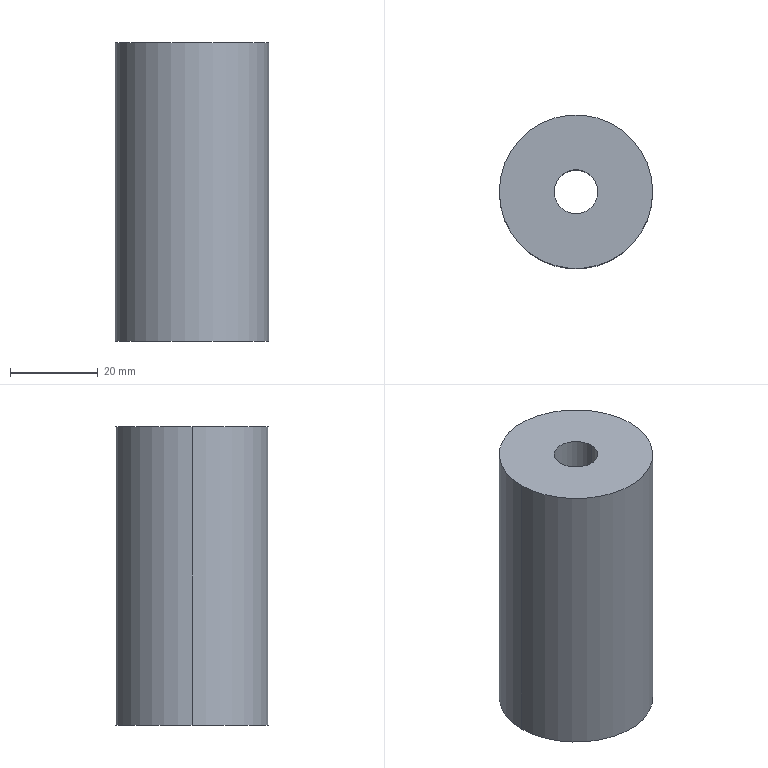Part | STEP file | 1 solid | 6 faces | box 35 x 35 x 68 mm | volume 60083 mm3 | cylinder 4 | plane 2 | commonest cylinder face diameters 10 x2 35 x2
STEP:
#1=CARTESIAN_POINT('',(0.,0.,0.));
#2=DIRECTION('',(0.,0.,1.));
#3=DIRECTION('',(1.,0.,0.));
#4=AXIS2_PLACEMENT_3D('',#1,#2,#3);
#5=CARTESIAN_POINT('',(194.63,-201.166,-34.));
#6=VERTEX_POINT('',#5);
#7=CARTESIAN_POINT('',(159.63,-201.166,-34.));
#8=VERTEX_POINT('',#7);
#9=CARTESIAN_POINT('',(177.13,-201.166,-34.));
#10=DIRECTION('',(0.,0.,1.));
#11=DIRECTION('',(1.,0.,0.));
#12=AXIS2_PLACEMENT_3D('',#9,#10,#11);
#13=CIRCLE('',#12,17.5);
#14=CARTESIAN_POINT('',(177.13,-201.166,0.));
#15=DIRECTION('',(0.,0.,1.));
#16=DIRECTION('',(1.,0.,0.));
#17=AXIS2_PLACEMENT_3D('',#14,#15,#16);
#18=CYLINDRICAL_SURFACE('',#17,17.5);
#19=CARTESIAN_POINT('',(0.,-34.));
#20=DIRECTION('',(1.,0.));
#21=VECTOR('',#20,1.);
#22=LINE('',#19,#21);
#23=(GEOMETRIC_REPRESENTATION_CONTEXT(2)PARAMETRIC_REPRESENTATION_CONTEXT()REPRESENTATION_CONTEXT('',''));
#24=DEFINITIONAL_REPRESENTATION('',(#22),#23);
#25=PCURVE('',#18,#24);
#26=CARTESIAN_POINT('',(177.13,-201.166,-34.));
#27=DIRECTION('',(0.,0.,1.));
#28=DIRECTION('',(1.,0.,0.));
#29=AXIS2_PLACEMENT_3D('',#26,#27,#28);
#30=PLANE('',#29);
#31=CARTESIAN_POINT('',(0.,0.));
#32=DIRECTION('',(1.,0.));
#33=AXIS2_PLACEMENT_2D('',#31,#32);
#34=CIRCLE('',#33,17.5);
#35=(GEOMETRIC_REPRESENTATION_CONTEXT(2)PARAMETRIC_REPRESENTATION_CONTEXT()REPRESENTATION_CONTEXT('',''));
#36=DEFINITIONAL_REPRESENTATION('',(#34),#35);
#37=PCURVE('',#30,#36);
#38=SURFACE_CURVE('',#13,(#25,#37),.PCURVE_S1.);
#39=EDGE_CURVE('',#6,#8,#38,.T.);
#40=ORIENTED_EDGE('',*,*,#39,.T.);
#41=CARTESIAN_POINT('',(159.63,-201.166,34.));
#42=VERTEX_POINT('',#41);
#43=CARTESIAN_POINT('',(159.63,-201.166,0.));
#44=DIRECTION('',(0.,0.,1.));
#45=VECTOR('',#44,1.);
#46=LINE('',#43,#45);
#47=CARTESIAN_POINT('',(3.142,0.));
#48=DIRECTION('',(0.,1.));
#49=VECTOR('',#48,1.);
#50=LINE('',#47,#49);
#51=(GEOMETRIC_REPRESENTATION_CONTEXT(2)PARAMETRIC_REPRESENTATION_CONTEXT()REPRESENTATION_CONTEXT('',''));
#52=DEFINITIONAL_REPRESENTATION('',(#50),#51);
#53=PCURVE('',#18,#52);
#54=CARTESIAN_POINT('',(177.13,-201.166,0.));
#55=DIRECTION('',(0.,0.,1.));
#56=DIRECTION('',(1.,0.,0.));
#57=AXIS2_PLACEMENT_3D('',#54,#55,#56);
#58=CYLINDRICAL_SURFACE('',#57,17.5);
#59=CARTESIAN_POINT('',(3.142,0.));
#60=DIRECTION('',(0.,1.));
#61=VECTOR('',#60,1.);
#62=LINE('',#59,#61);
#63=(GEOMETRIC_REPRESENTATION_CONTEXT(2)PARAMETRIC_REPRESENTATION_CONTEXT()REPRESENTATION_CONTEXT('',''));
#64=DEFINITIONAL_REPRESENTATION('',(#62),#63);
#65=PCURVE('',#58,#64);
#66=SURFACE_CURVE('',#46,(#53,#65),.PCURVE_S1.);
#67=EDGE_CURVE('',#8,#42,#66,.T.);
#68=ORIENTED_EDGE('',*,*,#67,.T.);
#69=CARTESIAN_POINT('',(194.63,-201.166,34.));
#70=VERTEX_POINT('',#69);
#71=CARTESIAN_POINT('',(177.13,-201.166,34.));
#72=DIRECTION('',(0.,0.,-1.));
#73=DIRECTION('',(1.,0.,0.));
#74=AXIS2_PLACEMENT_3D('',#71,#72,#73);
#75=CIRCLE('',#74,17.5);
#76=CARTESIAN_POINT('',(6.283,34.));
#77=DIRECTION('',(-1.,0.));
#78=VECTOR('',#77,1.);
#79=LINE('',#76,#78);
#80=(GEOMETRIC_REPRESENTATION_CONTEXT(2)PARAMETRIC_REPRESENTATION_CONTEXT()REPRESENTATION_CONTEXT('',''));
#81=DEFINITIONAL_REPRESENTATION('',(#79),#80);
#82=PCURVE('',#18,#81);
#83=CARTESIAN_POINT('',(177.13,-201.166,34.));
#84=DIRECTION('',(0.,0.,1.));
#85=DIRECTION('',(1.,0.,0.));
#86=AXIS2_PLACEMENT_3D('',#83,#84,#85);
#87=PLANE('',#86);
#88=CARTESIAN_POINT('',(17.5,0.));
#89=CARTESIAN_POINT('',(17.5,-30.311));
#90=CARTESIAN_POINT('',(-8.75,-15.155));
#91=CARTESIAN_POINT('',(-35.,0.));
#92=CARTESIAN_POINT('',(-8.75,15.155));
#93=CARTESIAN_POINT('',(17.5,30.311));
#94=CARTESIAN_POINT('',(17.5,0.));
#95=(BOUNDED_CURVE()B_SPLINE_CURVE(2,(#88,#89,#90,#91,#92,#93,#94),.UNSPECIFIED.,.T.,.F.)B_SPLINE_CURVE_WITH_KNOTS((1,2,2,2,2,1),(-2.094,0.,2.094,4.189,6.283,8.378),.UNSPECIFIED.)CURVE()GEOMETRIC_REPRESENTATION_ITEM()RATIONAL_B_SPLINE_CURVE((1.,0.5,1.,0.5,1.,0.5,1.))REPRESENTATION_ITEM(''));
#96=(GEOMETRIC_REPRESENTATION_CONTEXT(2)PARAMETRIC_REPRESENTATION_CONTEXT()REPRESENTATION_CONTEXT('',''));
#97=DEFINITIONAL_REPRESENTATION('',(#95),#96);
#98=PCURVE('',#87,#97);
#99=SURFACE_CURVE('',#75,(#82,#98),.PCURVE_S1.);
#100=EDGE_CURVE('',#42,#70,#99,.T.);
#101=ORIENTED_EDGE('',*,*,#100,.T.);
#102=CARTESIAN_POINT('',(194.63,-201.166,0.));
#103=DIRECTION('',(0.,0.,1.));
#104=VECTOR('',#103,1.);
#105=LINE('',#102,#104);
#106=CARTESIAN_POINT('',(0.,0.));
#107=DIRECTION('',(0.,1.));
#108=VECTOR('',#107,1.);
#109=LINE('',#106,#108);
#110=(GEOMETRIC_REPRESENTATION_CONTEXT(2)PARAMETRIC_REPRESENTATION_CONTEXT()REPRESENTATION_CONTEXT('',''));
#111=DEFINITIONAL_REPRESENTATION('',(#109),#110);
#112=PCURVE('',#18,#111);
#113=CARTESIAN_POINT('',(6.283,0.));
#114=DIRECTION('',(0.,1.));
#115=VECTOR('',#114,1.);
#116=LINE('',#113,#115);
#117=(GEOMETRIC_REPRESENTATION_CONTEXT(2)PARAMETRIC_REPRESENTATION_CONTEXT()REPRESENTATION_CONTEXT('',''));
#118=DEFINITIONAL_REPRESENTATION('',(#116),#117);
#119=PCURVE('',#58,#118);
#120=SURFACE_CURVE('',#105,(#112,#119),.PCURVE_S1.);
#121=EDGE_CURVE('',#6,#70,#120,.T.);
#122=ORIENTED_EDGE('',*,*,#121,.F.);
#123=EDGE_LOOP('',(#40,#68,#101,#122));
#124=FACE_BOUND('',#123,.T.);
#125=ADVANCED_FACE('',(#124),#18,.T.);
#126=CARTESIAN_POINT('',(182.13,-201.166,-34.));
#127=VERTEX_POINT('',#126);
#128=CARTESIAN_POINT('',(182.13,-201.166,34.));
#129=VERTEX_POINT('',#128);
#130=CARTESIAN_POINT('',(182.13,-201.166,0.));
#131=DIRECTION('',(0.,0.,1.));
#132=VECTOR('',#131,1.);
#133=LINE('',#130,#132);
#134=CARTESIAN_POINT('',(177.13,-201.166,0.));
#135=DIRECTION('',(0.,0.,1.));
#136=DIRECTION('',(1.,0.,0.));
#137=AXIS2_PLACEMENT_3D('',#134,#135,#136);
#138=CYLINDRICAL_SURFACE('',#137,5.);
#139=CARTESIAN_POINT('',(6.283,0.));
#140=DIRECTION('',(0.,1.));
#141=VECTOR('',#140,1.);
#142=LINE('',#139,#141);
#143=(GEOMETRIC_REPRESENTATION_CONTEXT(2)PARAMETRIC_REPRESENTATION_CONTEXT()REPRESENTATION_CONTEXT('',''));
#144=DEFINITIONAL_REPRESENTATION('',(#142),#143);
#145=PCURVE('',#138,#144);
#146=CARTESIAN_POINT('',(177.13,-201.166,0.));
#147=DIRECTION('',(0.,0.,1.));
#148=DIRECTION('',(1.,0.,0.));
#149=AXIS2_PLACEMENT_3D('',#146,#147,#148);
#150=CYLINDRICAL_SURFACE('',#149,5.);
#151=CARTESIAN_POINT('',(0.,0.));
#152=DIRECTION('',(0.,1.));
#153=VECTOR('',#152,1.);
#154=LINE('',#151,#153);
#155=(GEOMETRIC_REPRESENTATION_CONTEXT(2)PARAMETRIC_REPRESENTATION_CONTEXT()REPRESENTATION_CONTEXT('',''));
#156=DEFINITIONAL_REPRESENTATION('',(#154),#155);
#157=PCURVE('',#150,#156);
#158=SURFACE_CURVE('',#133,(#145,#157),.PCURVE_S1.);
#159=EDGE_CURVE('',#127,#129,#158,.T.);
#160=ORIENTED_EDGE('',*,*,#159,.T.);
#161=CARTESIAN_POINT('',(172.13,-201.166,34.));
#162=VERTEX_POINT('',#161);
#163=CARTESIAN_POINT('',(177.13,-201.166,34.));
#164=DIRECTION('',(0.,0.,-1.));
#165=DIRECTION('',(1.,0.,0.));
#166=AXIS2_PLACEMENT_3D('',#163,#164,#165);
#167=CIRCLE('',#166,5.);
#168=CARTESIAN_POINT('',(6.283,34.));
#169=DIRECTION('',(-1.,0.));
#170=VECTOR('',#169,1.);
#171=LINE('',#168,#170);
#172=(GEOMETRIC_REPRESENTATION_CONTEXT(2)PARAMETRIC_REPRESENTATION_CONTEXT()REPRESENTATION_CONTEXT('',''));
#173=DEFINITIONAL_REPRESENTATION('',(#171),#172);
#174=PCURVE('',#138,#173);
#175=CARTESIAN_POINT('',(5.,0.));
#176=CARTESIAN_POINT('',(5.,-8.66));
#177=CARTESIAN_POINT('',(-2.5,-4.33));
#178=CARTESIAN_POINT('',(-10.,0.));
#179=CARTESIAN_POINT('',(-2.5,4.33));
#180=CARTESIAN_POINT('',(5.,8.66));
#181=CARTESIAN_POINT('',(5.,0.));
#182=(BOUNDED_CURVE()B_SPLINE_CURVE(2,(#175,#176,#177,#178,#179,#180,#181),.UNSPECIFIED.,.T.,.F.)B_SPLINE_CURVE_WITH_KNOTS((1,2,2,2,2,1),(-2.094,0.,2.094,4.189,6.283,8.378),.UNSPECIFIED.)CURVE()GEOMETRIC_REPRESENTATION_ITEM()RATIONAL_B_SPLINE_CURVE((1.,0.5,1.,0.5,1.,0.5,1.))REPRESENTATION_ITEM(''));
#183=(GEOMETRIC_REPRESENTATION_CONTEXT(2)PARAMETRIC_REPRESENTATION_CONTEXT()REPRESENTATION_CONTEXT('',''));
#184=DEFINITIONAL_REPRESENTATION('',(#182),#183);
#185=PCURVE('',#87,#184);
#186=SURFACE_CURVE('',#167,(#174,#185),.PCURVE_S1.);
#187=EDGE_CURVE('',#129,#162,#186,.T.);
#188=ORIENTED_EDGE('',*,*,#187,.T.);
#189=CARTESIAN_POINT('',(172.13,-201.166,-34.));
#190=VERTEX_POINT('',#189);
#191=CARTESIAN_POINT('',(172.13,-201.166,0.));
#192=DIRECTION('',(0.,0.,1.));
#193=VECTOR('',#192,1.);
#194=LINE('',#191,#193);
#195=CARTESIAN_POINT('',(3.142,0.));
#196=DIRECTION('',(0.,1.));
#197=VECTOR('',#196,1.);
#198=LINE('',#195,#197);
#199=(GEOMETRIC_REPRESENTATION_CONTEXT(2)PARAMETRIC_REPRESENTATION_CONTEXT()REPRESENTATION_CONTEXT('',''));
#200=DEFINITIONAL_REPRESENTATION('',(#198),#199);
#201=PCURVE('',#138,#200);
#202=CARTESIAN_POINT('',(3.142,0.));
#203=DIRECTION('',(0.,1.));
#204=VECTOR('',#203,1.);
#205=LINE('',#202,#204);
#206=(GEOMETRIC_REPRESENTATION_CONTEXT(2)PARAMETRIC_REPRESENTATION_CONTEXT()REPRESENTATION_CONTEXT('',''));
#207=DEFINITIONAL_REPRESENTATION('',(#205),#206);
#208=PCURVE('',#150,#207);
#209=SURFACE_CURVE('',#194,(#201,#208),.PCURVE_S1.);
#210=EDGE_CURVE('',#190,#162,#209,.T.);
#211=ORIENTED_EDGE('',*,*,#210,.F.);
#212=CARTESIAN_POINT('',(177.13,-201.166,-34.));
#213=DIRECTION('',(0.,0.,-1.));
#214=DIRECTION('',(1.,0.,0.));
#215=AXIS2_PLACEMENT_3D('',#212,#213,#214);
#216=CIRCLE('',#215,5.);
#217=CARTESIAN_POINT('',(6.283,-34.));
#218=DIRECTION('',(-1.,0.));
#219=VECTOR('',#218,1.);
#220=LINE('',#217,#219);
#221=(GEOMETRIC_REPRESENTATION_CONTEXT(2)PARAMETRIC_REPRESENTATION_CONTEXT()REPRESENTATION_CONTEXT('',''));
#222=DEFINITIONAL_REPRESENTATION('',(#220),#221);
#223=PCURVE('',#138,#222);
#224=CARTESIAN_POINT('',(5.,0.));
#225=CARTESIAN_POINT('',(5.,-8.66));
#226=CARTESIAN_POINT('',(-2.5,-4.33));
#227=CARTESIAN_POINT('',(-10.,0.));
#228=CARTESIAN_POINT('',(-2.5,4.33));
#229=CARTESIAN_POINT('',(5.,8.66));
#230=CARTESIAN_POINT('',(5.,0.));
#231=(BOUNDED_CURVE()B_SPLINE_CURVE(2,(#224,#225,#226,#227,#228,#229,#230),.UNSPECIFIED.,.T.,.F.)B_SPLINE_CURVE_WITH_KNOTS((1,2,2,2,2,1),(-2.094,0.,2.094,4.189,6.283,8.378),.UNSPECIFIED.)CURVE()GEOMETRIC_REPRESENTATION_ITEM()RATIONAL_B_SPLINE_CURVE((1.,0.5,1.,0.5,1.,0.5,1.))REPRESENTATION_ITEM(''));
#232=(GEOMETRIC_REPRESENTATION_CONTEXT(2)PARAMETRIC_REPRESENTATION_CONTEXT()REPRESENTATION_CONTEXT('',''));
#233=DEFINITIONAL_REPRESENTATION('',(#231),#232);
#234=PCURVE('',#30,#233);
#235=SURFACE_CURVE('',#216,(#223,#234),.PCURVE_S1.);
#236=EDGE_CURVE('',#127,#190,#235,.T.);
#237=ORIENTED_EDGE('',*,*,#236,.F.);
#238=EDGE_LOOP('',(#160,#188,#211,#237));
#239=FACE_BOUND('',#238,.F.);
#240=ADVANCED_FACE('',(#239),#138,.F.);
#241=ORIENTED_EDGE('',*,*,#67,.F.);
#242=CARTESIAN_POINT('',(177.13,-201.166,-34.));
#243=DIRECTION('',(0.,0.,1.));
#244=DIRECTION('',(1.,0.,0.));
#245=AXIS2_PLACEMENT_3D('',#242,#243,#244);
#246=CIRCLE('',#245,17.5);
#247=CARTESIAN_POINT('',(0.,-34.));
#248=DIRECTION('',(1.,0.));
#249=VECTOR('',#248,1.);
#250=LINE('',#247,#249);
#251=(GEOMETRIC_REPRESENTATION_CONTEXT(2)PARAMETRIC_REPRESENTATION_CONTEXT()REPRESENTATION_CONTEXT('',''));
#252=DEFINITIONAL_REPRESENTATION('',(#250),#251);
#253=PCURVE('',#58,#252);
#254=CARTESIAN_POINT('',(0.,0.));
#255=DIRECTION('',(1.,0.));
#256=AXIS2_PLACEMENT_2D('',#254,#255);
#257=CIRCLE('',#256,17.5);
#258=(GEOMETRIC_REPRESENTATION_CONTEXT(2)PARAMETRIC_REPRESENTATION_CONTEXT()REPRESENTATION_CONTEXT('',''));
#259=DEFINITIONAL_REPRESENTATION('',(#257),#258);
#260=PCURVE('',#30,#259);
#261=SURFACE_CURVE('',#246,(#253,#260),.PCURVE_S1.);
#262=EDGE_CURVE('',#8,#6,#261,.T.);
#263=ORIENTED_EDGE('',*,*,#262,.T.);
#264=ORIENTED_EDGE('',*,*,#121,.T.);
#265=CARTESIAN_POINT('',(177.13,-201.166,34.));
#266=DIRECTION('',(0.,0.,-1.));
#267=DIRECTION('',(1.,0.,0.));
#268=AXIS2_PLACEMENT_3D('',#265,#266,#267);
#269=CIRCLE('',#268,17.5);
#270=CARTESIAN_POINT('',(6.283,34.));
#271=DIRECTION('',(-1.,0.));
#272=VECTOR('',#271,1.);
#273=LINE('',#270,#272);
#274=(GEOMETRIC_REPRESENTATION_CONTEXT(2)PARAMETRIC_REPRESENTATION_CONTEXT()REPRESENTATION_CONTEXT('',''));
#275=DEFINITIONAL_REPRESENTATION('',(#273),#274);
#276=PCURVE('',#58,#275);
#277=CARTESIAN_POINT('',(17.5,0.));
#278=CARTESIAN_POINT('',(17.5,-30.311));
#279=CARTESIAN_POINT('',(-8.75,-15.155));
#280=CARTESIAN_POINT('',(-35.,0.));
#281=CARTESIAN_POINT('',(-8.75,15.155));
#282=CARTESIAN_POINT('',(17.5,30.311));
#283=CARTESIAN_POINT('',(17.5,0.));
#284=(BOUNDED_CURVE()B_SPLINE_CURVE(2,(#277,#278,#279,#280,#281,#282,#283),.UNSPECIFIED.,.T.,.F.)B_SPLINE_CURVE_WITH_KNOTS((1,2,2,2,2,1),(-2.094,0.,2.094,4.189,6.283,8.378),.UNSPECIFIED.)CURVE()GEOMETRIC_REPRESENTATION_ITEM()RATIONAL_B_SPLINE_CURVE((1.,0.5,1.,0.5,1.,0.5,1.))REPRESENTATION_ITEM(''));
#285=(GEOMETRIC_REPRESENTATION_CONTEXT(2)PARAMETRIC_REPRESENTATION_CONTEXT()REPRESENTATION_CONTEXT('',''));
#286=DEFINITIONAL_REPRESENTATION('',(#284),#285);
#287=PCURVE('',#87,#286);
#288=SURFACE_CURVE('',#269,(#276,#287),.PCURVE_S1.);
#289=EDGE_CURVE('',#70,#42,#288,.T.);
#290=ORIENTED_EDGE('',*,*,#289,.T.);
#291=EDGE_LOOP('',(#241,#263,#264,#290));
#292=FACE_BOUND('',#291,.T.);
#293=ADVANCED_FACE('',(#292),#58,.T.);
#294=ORIENTED_EDGE('',*,*,#289,.F.);
#295=ORIENTED_EDGE('',*,*,#100,.F.);
#296=EDGE_LOOP('',(#294,#295));
#297=FACE_BOUND('',#296,.T.);
#298=ORIENTED_EDGE('',*,*,#187,.T.);
#299=CARTESIAN_POINT('',(177.13,-201.166,34.));
#300=DIRECTION('',(0.,0.,-1.));
#301=DIRECTION('',(1.,0.,0.));
#302=AXIS2_PLACEMENT_3D('',#299,#300,#301);
#303=CIRCLE('',#302,5.);
#304=CARTESIAN_POINT('',(5.,0.));
#305=CARTESIAN_POINT('',(5.,-8.66));
#306=CARTESIAN_POINT('',(-2.5,-4.33));
#307=CARTESIAN_POINT('',(-10.,0.));
#308=CARTESIAN_POINT('',(-2.5,4.33));
#309=CARTESIAN_POINT('',(5.,8.66));
#310=CARTESIAN_POINT('',(5.,0.));
#311=(BOUNDED_CURVE()B_SPLINE_CURVE(2,(#304,#305,#306,#307,#308,#309,#310),.UNSPECIFIED.,.T.,.F.)B_SPLINE_CURVE_WITH_KNOTS((1,2,2,2,2,1),(-2.094,0.,2.094,4.189,6.283,8.378),.UNSPECIFIED.)CURVE()GEOMETRIC_REPRESENTATION_ITEM()RATIONAL_B_SPLINE_CURVE((1.,0.5,1.,0.5,1.,0.5,1.))REPRESENTATION_ITEM(''));
#312=(GEOMETRIC_REPRESENTATION_CONTEXT(2)PARAMETRIC_REPRESENTATION_CONTEXT()REPRESENTATION_CONTEXT('',''));
#313=DEFINITIONAL_REPRESENTATION('',(#311),#312);
#314=PCURVE('',#87,#313);
#315=CARTESIAN_POINT('',(6.283,34.));
#316=DIRECTION('',(-1.,0.));
#317=VECTOR('',#316,1.);
#318=LINE('',#315,#317);
#319=(GEOMETRIC_REPRESENTATION_CONTEXT(2)PARAMETRIC_REPRESENTATION_CONTEXT()REPRESENTATION_CONTEXT('',''));
#320=DEFINITIONAL_REPRESENTATION('',(#318),#319);
#321=PCURVE('',#150,#320);
#322=SURFACE_CURVE('',#303,(#314,#321),.PCURVE_S1.);
#323=EDGE_CURVE('',#162,#129,#322,.T.);
#324=ORIENTED_EDGE('',*,*,#323,.T.);
#325=EDGE_LOOP('',(#298,#324));
#326=FACE_BOUND('',#325,.T.);
#327=ADVANCED_FACE('',(#297,#326),#87,.T.);
#328=ORIENTED_EDGE('',*,*,#39,.F.);
#329=ORIENTED_EDGE('',*,*,#262,.F.);
#330=EDGE_LOOP('',(#328,#329));
#331=FACE_BOUND('',#330,.T.);
#332=ORIENTED_EDGE('',*,*,#236,.F.);
#333=CARTESIAN_POINT('',(177.13,-201.166,-34.));
#334=DIRECTION('',(0.,0.,-1.));
#335=DIRECTION('',(1.,0.,0.));
#336=AXIS2_PLACEMENT_3D('',#333,#334,#335);
#337=CIRCLE('',#336,5.);
#338=CARTESIAN_POINT('',(5.,0.));
#339=CARTESIAN_POINT('',(5.,-8.66));
#340=CARTESIAN_POINT('',(-2.5,-4.33));
#341=CARTESIAN_POINT('',(-10.,0.));
#342=CARTESIAN_POINT('',(-2.5,4.33));
#343=CARTESIAN_POINT('',(5.,8.66));
#344=CARTESIAN_POINT('',(5.,0.));
#345=(BOUNDED_CURVE()B_SPLINE_CURVE(2,(#338,#339,#340,#341,#342,#343,#344),.UNSPECIFIED.,.T.,.F.)B_SPLINE_CURVE_WITH_KNOTS((1,2,2,2,2,1),(-2.094,0.,2.094,4.189,6.283,8.378),.UNSPECIFIED.)CURVE()GEOMETRIC_REPRESENTATION_ITEM()RATIONAL_B_SPLINE_CURVE((1.,0.5,1.,0.5,1.,0.5,1.))REPRESENTATION_ITEM(''));
#346=(GEOMETRIC_REPRESENTATION_CONTEXT(2)PARAMETRIC_REPRESENTATION_CONTEXT()REPRESENTATION_CONTEXT('',''));
#347=DEFINITIONAL_REPRESENTATION('',(#345),#346);
#348=PCURVE('',#30,#347);
#349=CARTESIAN_POINT('',(6.283,-34.));
#350=DIRECTION('',(-1.,0.));
#351=VECTOR('',#350,1.);
#352=LINE('',#349,#351);
#353=(GEOMETRIC_REPRESENTATION_CONTEXT(2)PARAMETRIC_REPRESENTATION_CONTEXT()REPRESENTATION_CONTEXT('',''));
#354=DEFINITIONAL_REPRESENTATION('',(#352),#353);
#355=PCURVE('',#150,#354);
#356=SURFACE_CURVE('',#337,(#348,#355),.PCURVE_S1.);
#357=EDGE_CURVE('',#190,#127,#356,.T.);
#358=ORIENTED_EDGE('',*,*,#357,.F.);
#359=EDGE_LOOP('',(#332,#358));
#360=FACE_BOUND('',#359,.T.);
#361=ADVANCED_FACE('',(#331,#360),#30,.F.);
#362=ORIENTED_EDGE('',*,*,#323,.T.);
#363=ORIENTED_EDGE('',*,*,#159,.F.);
#364=ORIENTED_EDGE('',*,*,#357,.F.);
#365=ORIENTED_EDGE('',*,*,#210,.T.);
#366=EDGE_LOOP('',(#362,#363,#364,#365));
#367=FACE_BOUND('',#366,.F.);
#368=ADVANCED_FACE('',(#367),#150,.F.);
#369=CLOSED_SHELL('',(#125,#240,#293,#327,#361,#368));
#370=MANIFOLD_SOLID_BREP('',#369);
#371=(LENGTH_UNIT()NAMED_UNIT(*)SI_UNIT(.MILLI.,.METRE.));
#372=UNCERTAINTY_MEASURE_WITH_UNIT(LENGTH_MEASURE(0.0000001),#371,'','');
#373=(NAMED_UNIT(*)PLANE_ANGLE_UNIT()SI_UNIT($,.RADIAN.));
#374=(NAMED_UNIT(*)SI_UNIT($,.STERADIAN.)SOLID_ANGLE_UNIT());
#375=(GEOMETRIC_REPRESENTATION_CONTEXT(3)GLOBAL_UNCERTAINTY_ASSIGNED_CONTEXT((#372))GLOBAL_UNIT_ASSIGNED_CONTEXT((#371,#373,#374))REPRESENTATION_CONTEXT('',''));
#376=ADVANCED_BREP_SHAPE_REPRESENTATION('',(#4,#370),#375);